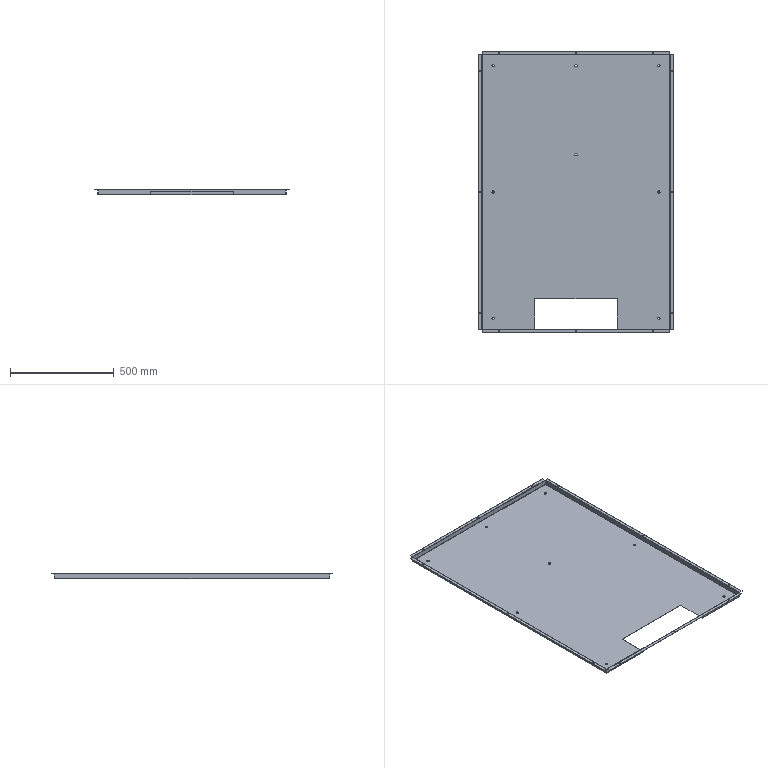Part | SolidWorks | features ICE 4, EdgeFlange 2, FlatPattern 1, SMBaseFlange 1, SheetMetal 1 | 1 solid | 150 faces | box 940 x 1360 x 25 mm | volume 1313898 mm3 | plane 78 | cylinder 64 | spline 8 | commonest cylinder face diameters 7 x30 11 x16 0.4 x9 2.4 x9